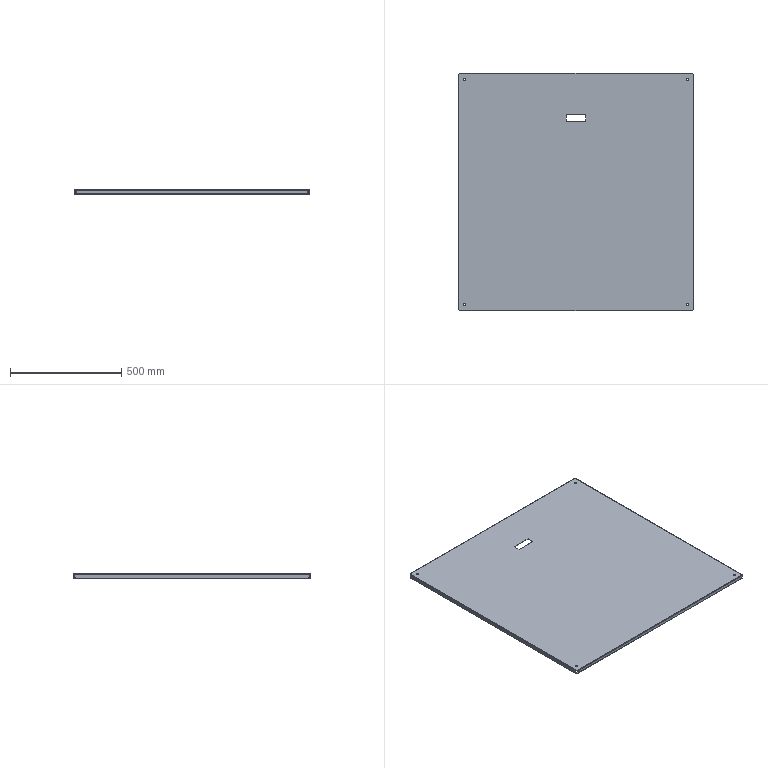Part | SolidWorks | features BaseBody 1 | 1 solid | 50 faces | box 1056 x 1066 x 18 mm | volume 1814668 mm3 | plane 30 | cylinder 20 | commonest cylinder face diameters 9 x8 1.473 x6 4.473 x6